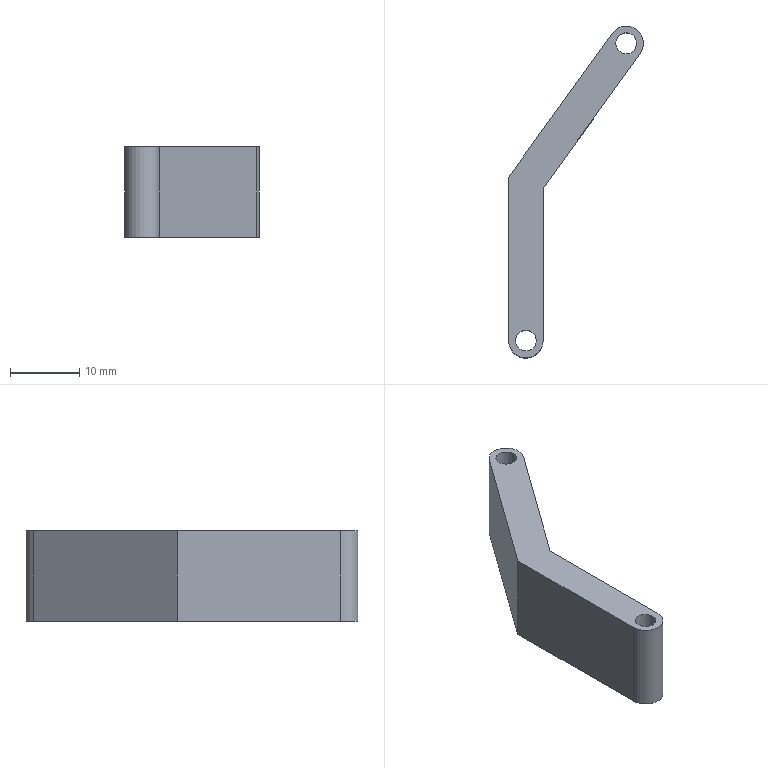Part | SolidWorks | features BaseBody 1 | 1 solid | 12 faces | box 19.494 x 47.938 x 13 mm | volume 3166 mm3 | cylinder 6 | plane 6 | commonest cylinder face diameters 3 x4 5 x2
STEP:
#1=CARTESIAN_POINT('',(-4.,-22.,13.));
#2=VERTEX_POINT('',#1);
#3=CARTESIAN_POINT('',(-1.,-22.,13.));
#4=VERTEX_POINT('',#3);
#5=CARTESIAN_POINT('',(-2.5,-22.,13.));
#6=DIRECTION('',(0.,0.,1.));
#7=DIRECTION('',(1.,0.,0.));
#8=AXIS2_PLACEMENT_3D('',#5,#6,#7);
#9=CIRCLE('',#8,1.5);
#10=EDGE_CURVE('',#2,#4,#9,.T.);
#11=ORIENTED_EDGE('',*,*,#10,.T.);
#12=CARTESIAN_POINT('',(-1.,-22.,0.));
#13=VERTEX_POINT('',#12);
#14=CARTESIAN_POINT('',(-1.,-22.,13.));
#15=DIRECTION('',(0.,0.,-1.));
#16=VECTOR('',#15,1000.);
#17=LINE('',#14,#16);
#18=EDGE_CURVE('',#4,#13,#17,.T.);
#19=ORIENTED_EDGE('',*,*,#18,.T.);
#20=CARTESIAN_POINT('',(-4.,-22.,0.));
#21=VERTEX_POINT('',#20);
#22=CARTESIAN_POINT('',(-2.5,-22.,0.));
#23=DIRECTION('',(0.,0.,1.));
#24=DIRECTION('',(1.,0.,0.));
#25=AXIS2_PLACEMENT_3D('',#22,#23,#24);
#26=CIRCLE('',#25,1.5);
#27=EDGE_CURVE('',#21,#13,#26,.T.);
#28=ORIENTED_EDGE('',*,*,#27,.F.);
#29=CARTESIAN_POINT('',(-4.,-22.,13.));
#30=DIRECTION('',(0.,0.,-1.));
#31=VECTOR('',#30,1000.);
#32=LINE('',#29,#31);
#33=EDGE_CURVE('',#2,#21,#32,.T.);
#34=ORIENTED_EDGE('',*,*,#33,.F.);
#35=EDGE_LOOP('',(#11,#19,#28,#34));
#36=FACE_OUTER_BOUND('',#35,.T.);
#37=CARTESIAN_POINT('',(-2.5,-22.,13.));
#38=DIRECTION('',(0.,0.,-1.));
#39=DIRECTION('',(-1.,0.,0.));
#40=AXIS2_PLACEMENT_3D('',#37,#38,#39);
#41=CYLINDRICAL_SURFACE('',#40,1.5);
#42=ADVANCED_FACE('',(#36),#41,.F.);
#43=CARTESIAN_POINT('',(10.494,20.938,13.));
#44=VERTEX_POINT('',#43);
#45=CARTESIAN_POINT('',(13.494,20.938,13.));
#46=VERTEX_POINT('',#45);
#47=CARTESIAN_POINT('',(11.994,20.938,13.));
#48=DIRECTION('',(0.,0.,1.));
#49=DIRECTION('',(1.,0.,0.));
#50=AXIS2_PLACEMENT_3D('',#47,#48,#49);
#51=CIRCLE('',#50,1.5);
#52=EDGE_CURVE('',#44,#46,#51,.T.);
#53=ORIENTED_EDGE('',*,*,#52,.T.);
#54=CARTESIAN_POINT('',(13.494,20.938,0.));
#55=VERTEX_POINT('',#54);
#56=CARTESIAN_POINT('',(13.494,20.938,13.));
#57=DIRECTION('',(0.,0.,-1.));
#58=VECTOR('',#57,1000.);
#59=LINE('',#56,#58);
#60=EDGE_CURVE('',#46,#55,#59,.T.);
#61=ORIENTED_EDGE('',*,*,#60,.T.);
#62=CARTESIAN_POINT('',(10.494,20.938,0.));
#63=VERTEX_POINT('',#62);
#64=CARTESIAN_POINT('',(11.994,20.938,0.));
#65=DIRECTION('',(0.,0.,1.));
#66=DIRECTION('',(1.,0.,0.));
#67=AXIS2_PLACEMENT_3D('',#64,#65,#66);
#68=CIRCLE('',#67,1.5);
#69=EDGE_CURVE('',#63,#55,#68,.T.);
#70=ORIENTED_EDGE('',*,*,#69,.F.);
#71=CARTESIAN_POINT('',(10.494,20.938,13.));
#72=DIRECTION('',(0.,0.,-1.));
#73=VECTOR('',#72,1000.);
#74=LINE('',#71,#73);
#75=EDGE_CURVE('',#44,#63,#74,.T.);
#76=ORIENTED_EDGE('',*,*,#75,.F.);
#77=EDGE_LOOP('',(#53,#61,#70,#76));
#78=FACE_OUTER_BOUND('',#77,.T.);
#79=CARTESIAN_POINT('',(11.994,20.938,13.));
#80=DIRECTION('',(0.,0.,-1.));
#81=DIRECTION('',(-1.,0.,0.));
#82=AXIS2_PLACEMENT_3D('',#79,#80,#81);
#83=CYLINDRICAL_SURFACE('',#82,1.5);
#84=ADVANCED_FACE('',(#78),#83,.F.);
#85=ORIENTED_EDGE('',*,*,#52,.F.);
#86=CARTESIAN_POINT('',(11.994,20.938,13.));
#87=DIRECTION('',(0.,0.,1.));
#88=DIRECTION('',(1.,0.,0.));
#89=AXIS2_PLACEMENT_3D('',#86,#87,#88);
#90=CIRCLE('',#89,1.5);
#91=EDGE_CURVE('',#46,#44,#90,.T.);
#92=ORIENTED_EDGE('',*,*,#91,.F.);
#93=EDGE_LOOP('',(#85,#92));
#94=FACE_BOUND('',#93,.T.);
#95=CARTESIAN_POINT('',(0.,0.,13.));
#96=VERTEX_POINT('',#95);
#97=CARTESIAN_POINT('',(14.023,19.477,13.));
#98=VERTEX_POINT('',#97);
#99=CARTESIAN_POINT('',(0.,0.,13.));
#100=DIRECTION('',(0.5843,0.8115,0.));
#101=VECTOR('',#100,1000.);
#102=LINE('',#99,#101);
#103=EDGE_CURVE('',#96,#98,#102,.T.);
#104=ORIENTED_EDGE('',*,*,#103,.T.);
#105=CARTESIAN_POINT('',(9.966,22.398,13.));
#106=VERTEX_POINT('',#105);
#107=CARTESIAN_POINT('',(11.994,20.938,13.));
#108=DIRECTION('',(0.,0.,1.));
#109=DIRECTION('',(1.,0.,0.));
#110=AXIS2_PLACEMENT_3D('',#107,#108,#109);
#111=CIRCLE('',#110,2.5);
#112=EDGE_CURVE('',#98,#106,#111,.T.);
#113=ORIENTED_EDGE('',*,*,#112,.T.);
#114=CARTESIAN_POINT('',(-5.,1.613,13.));
#115=VERTEX_POINT('',#114);
#116=CARTESIAN_POINT('',(-5.,1.613,13.));
#117=DIRECTION('',(-0.5843,-0.8115,0.));
#118=VECTOR('',#117,1000.);
#119=LINE('',#116,#118);
#120=EDGE_CURVE('',#106,#115,#119,.T.);
#121=ORIENTED_EDGE('',*,*,#120,.T.);
#122=CARTESIAN_POINT('',(-5.,-22.,13.));
#123=VERTEX_POINT('',#122);
#124=CARTESIAN_POINT('',(-5.,1.613,13.));
#125=DIRECTION('',(0.,-1.,0.));
#126=VECTOR('',#125,1000.);
#127=LINE('',#124,#126);
#128=EDGE_CURVE('',#115,#123,#127,.T.);
#129=ORIENTED_EDGE('',*,*,#128,.T.);
#130=CARTESIAN_POINT('',(0.,-22.,13.));
#131=VERTEX_POINT('',#130);
#132=CARTESIAN_POINT('',(-2.5,-22.,13.));
#133=DIRECTION('',(0.,0.,1.));
#134=DIRECTION('',(-1.,0.,0.));
#135=AXIS2_PLACEMENT_3D('',#132,#133,#134);
#136=CIRCLE('',#135,2.5);
#137=EDGE_CURVE('',#123,#131,#136,.T.);
#138=ORIENTED_EDGE('',*,*,#137,.T.);
#139=CARTESIAN_POINT('',(0.,0.,13.));
#140=DIRECTION('',(0.,1.,0.));
#141=VECTOR('',#140,1000.);
#142=LINE('',#139,#141);
#143=EDGE_CURVE('',#131,#96,#142,.T.);
#144=ORIENTED_EDGE('',*,*,#143,.T.);
#145=EDGE_LOOP('',(#104,#113,#121,#129,#138,#144));
#146=FACE_OUTER_BOUND('',#145,.T.);
#147=ORIENTED_EDGE('',*,*,#10,.F.);
#148=CARTESIAN_POINT('',(-2.5,-22.,13.));
#149=DIRECTION('',(0.,0.,1.));
#150=DIRECTION('',(1.,0.,0.));
#151=AXIS2_PLACEMENT_3D('',#148,#149,#150);
#152=CIRCLE('',#151,1.5);
#153=EDGE_CURVE('',#4,#2,#152,.T.);
#154=ORIENTED_EDGE('',*,*,#153,.F.);
#155=EDGE_LOOP('',(#147,#154));
#156=FACE_BOUND('',#155,.T.);
#157=CARTESIAN_POINT('',(11.994,20.938,13.));
#158=DIRECTION('',(0.,0.,1.));
#159=DIRECTION('',(1.,0.,0.));
#160=AXIS2_PLACEMENT_3D('',#157,#158,#159);
#161=PLANE('',#160);
#162=ADVANCED_FACE('',(#94,#146,#156),#161,.T.);
#163=CARTESIAN_POINT('',(0.,0.,0.));
#164=VERTEX_POINT('',#163);
#165=CARTESIAN_POINT('',(14.023,19.477,0.));
#166=VERTEX_POINT('',#165);
#167=CARTESIAN_POINT('',(0.,0.,0.));
#168=DIRECTION('',(0.5843,0.8115,0.));
#169=VECTOR('',#168,1000.);
#170=LINE('',#167,#169);
#171=EDGE_CURVE('',#164,#166,#170,.T.);
#172=ORIENTED_EDGE('',*,*,#171,.F.);
#173=CARTESIAN_POINT('',(0.,-22.,0.));
#174=VERTEX_POINT('',#173);
#175=CARTESIAN_POINT('',(0.,0.,0.));
#176=DIRECTION('',(0.,1.,0.));
#177=VECTOR('',#176,1000.);
#178=LINE('',#175,#177);
#179=EDGE_CURVE('',#174,#164,#178,.T.);
#180=ORIENTED_EDGE('',*,*,#179,.F.);
#181=CARTESIAN_POINT('',(-5.,-22.,0.));
#182=VERTEX_POINT('',#181);
#183=CARTESIAN_POINT('',(-2.5,-22.,0.));
#184=DIRECTION('',(0.,0.,1.));
#185=DIRECTION('',(-1.,0.,0.));
#186=AXIS2_PLACEMENT_3D('',#183,#184,#185);
#187=CIRCLE('',#186,2.5);
#188=EDGE_CURVE('',#182,#174,#187,.T.);
#189=ORIENTED_EDGE('',*,*,#188,.F.);
#190=CARTESIAN_POINT('',(-5.,1.613,0.));
#191=VERTEX_POINT('',#190);
#192=CARTESIAN_POINT('',(-5.,1.613,0.));
#193=DIRECTION('',(0.,-1.,0.));
#194=VECTOR('',#193,1000.);
#195=LINE('',#192,#194);
#196=EDGE_CURVE('',#191,#182,#195,.T.);
#197=ORIENTED_EDGE('',*,*,#196,.F.);
#198=CARTESIAN_POINT('',(9.966,22.398,0.));
#199=VERTEX_POINT('',#198);
#200=CARTESIAN_POINT('',(-5.,1.613,0.));
#201=DIRECTION('',(-0.5843,-0.8115,0.));
#202=VECTOR('',#201,1000.);
#203=LINE('',#200,#202);
#204=EDGE_CURVE('',#199,#191,#203,.T.);
#205=ORIENTED_EDGE('',*,*,#204,.F.);
#206=CARTESIAN_POINT('',(11.994,20.938,0.));
#207=DIRECTION('',(0.,0.,1.));
#208=DIRECTION('',(1.,0.,0.));
#209=AXIS2_PLACEMENT_3D('',#206,#207,#208);
#210=CIRCLE('',#209,2.5);
#211=EDGE_CURVE('',#166,#199,#210,.T.);
#212=ORIENTED_EDGE('',*,*,#211,.F.);
#213=EDGE_LOOP('',(#172,#180,#189,#197,#205,#212));
#214=FACE_OUTER_BOUND('',#213,.T.);
#215=ORIENTED_EDGE('',*,*,#69,.T.);
#216=CARTESIAN_POINT('',(11.994,20.938,0.));
#217=DIRECTION('',(0.,0.,1.));
#218=DIRECTION('',(1.,0.,0.));
#219=AXIS2_PLACEMENT_3D('',#216,#217,#218);
#220=CIRCLE('',#219,1.5);
#221=EDGE_CURVE('',#55,#63,#220,.T.);
#222=ORIENTED_EDGE('',*,*,#221,.T.);
#223=EDGE_LOOP('',(#215,#222));
#224=FACE_BOUND('',#223,.T.);
#225=ORIENTED_EDGE('',*,*,#27,.T.);
#226=CARTESIAN_POINT('',(-2.5,-22.,0.));
#227=DIRECTION('',(0.,0.,1.));
#228=DIRECTION('',(1.,0.,0.));
#229=AXIS2_PLACEMENT_3D('',#226,#227,#228);
#230=CIRCLE('',#229,1.5);
#231=EDGE_CURVE('',#13,#21,#230,.T.);
#232=ORIENTED_EDGE('',*,*,#231,.T.);
#233=EDGE_LOOP('',(#225,#232));
#234=FACE_BOUND('',#233,.T.);
#235=CARTESIAN_POINT('',(11.994,20.938,0.));
#236=DIRECTION('',(0.,0.,1.));
#237=DIRECTION('',(1.,0.,0.));
#238=AXIS2_PLACEMENT_3D('',#235,#236,#237);
#239=PLANE('',#238);
#240=ADVANCED_FACE('',(#214,#224,#234),#239,.F.);
#241=ORIENTED_EDGE('',*,*,#171,.T.);
#242=CARTESIAN_POINT('',(14.023,19.477,13.));
#243=DIRECTION('',(0.,0.,-1.));
#244=VECTOR('',#243,1000.);
#245=LINE('',#242,#244);
#246=EDGE_CURVE('',#98,#166,#245,.T.);
#247=ORIENTED_EDGE('',*,*,#246,.F.);
#248=ORIENTED_EDGE('',*,*,#103,.F.);
#249=CARTESIAN_POINT('',(0.,0.,13.));
#250=DIRECTION('',(0.,0.,-1.));
#251=VECTOR('',#250,1000.);
#252=LINE('',#249,#251);
#253=EDGE_CURVE('',#96,#164,#252,.T.);
#254=ORIENTED_EDGE('',*,*,#253,.T.);
#255=EDGE_LOOP('',(#241,#247,#248,#254));
#256=FACE_OUTER_BOUND('',#255,.T.);
#257=CARTESIAN_POINT('',(0.,0.,13.));
#258=DIRECTION('',(-0.8115,0.5843,0.));
#259=DIRECTION('',(-0.5843,-0.8115,0.));
#260=AXIS2_PLACEMENT_3D('',#257,#258,#259);
#261=PLANE('',#260);
#262=ADVANCED_FACE('',(#256),#261,.F.);
#263=ORIENTED_EDGE('',*,*,#211,.T.);
#264=CARTESIAN_POINT('',(9.966,22.398,13.));
#265=DIRECTION('',(0.,0.,-1.));
#266=VECTOR('',#265,1000.);
#267=LINE('',#264,#266);
#268=EDGE_CURVE('',#106,#199,#267,.T.);
#269=ORIENTED_EDGE('',*,*,#268,.F.);
#270=ORIENTED_EDGE('',*,*,#112,.F.);
#271=ORIENTED_EDGE('',*,*,#246,.T.);
#272=EDGE_LOOP('',(#263,#269,#270,#271));
#273=FACE_OUTER_BOUND('',#272,.T.);
#274=CARTESIAN_POINT('',(11.994,20.938,13.));
#275=DIRECTION('',(0.,0.,-1.));
#276=DIRECTION('',(-1.,0.,0.));
#277=AXIS2_PLACEMENT_3D('',#274,#275,#276);
#278=CYLINDRICAL_SURFACE('',#277,2.5);
#279=ADVANCED_FACE('',(#273),#278,.T.);
#280=ORIENTED_EDGE('',*,*,#204,.T.);
#281=CARTESIAN_POINT('',(-5.,1.613,13.));
#282=DIRECTION('',(0.,0.,-1.));
#283=VECTOR('',#282,1000.);
#284=LINE('',#281,#283);
#285=EDGE_CURVE('',#115,#191,#284,.T.);
#286=ORIENTED_EDGE('',*,*,#285,.F.);
#287=ORIENTED_EDGE('',*,*,#120,.F.);
#288=ORIENTED_EDGE('',*,*,#268,.T.);
#289=EDGE_LOOP('',(#280,#286,#287,#288));
#290=FACE_OUTER_BOUND('',#289,.T.);
#291=CARTESIAN_POINT('',(-5.,1.613,13.));
#292=DIRECTION('',(0.8115,-0.5843,0.));
#293=DIRECTION('',(0.5843,0.8115,0.));
#294=AXIS2_PLACEMENT_3D('',#291,#292,#293);
#295=PLANE('',#294);
#296=ADVANCED_FACE('',(#290),#295,.F.);
#297=ORIENTED_EDGE('',*,*,#196,.T.);
#298=CARTESIAN_POINT('',(-5.,-22.,13.));
#299=DIRECTION('',(0.,0.,-1.));
#300=VECTOR('',#299,1000.);
#301=LINE('',#298,#300);
#302=EDGE_CURVE('',#123,#182,#301,.T.);
#303=ORIENTED_EDGE('',*,*,#302,.F.);
#304=ORIENTED_EDGE('',*,*,#128,.F.);
#305=ORIENTED_EDGE('',*,*,#285,.T.);
#306=EDGE_LOOP('',(#297,#303,#304,#305));
#307=FACE_OUTER_BOUND('',#306,.T.);
#308=CARTESIAN_POINT('',(-5.,1.613,13.));
#309=DIRECTION('',(1.,0.,0.));
#310=DIRECTION('',(0.,1.,0.));
#311=AXIS2_PLACEMENT_3D('',#308,#309,#310);
#312=PLANE('',#311);
#313=ADVANCED_FACE('',(#307),#312,.F.);
#314=ORIENTED_EDGE('',*,*,#188,.T.);
#315=CARTESIAN_POINT('',(0.,-22.,13.));
#316=DIRECTION('',(0.,0.,-1.));
#317=VECTOR('',#316,1000.);
#318=LINE('',#315,#317);
#319=EDGE_CURVE('',#131,#174,#318,.T.);
#320=ORIENTED_EDGE('',*,*,#319,.F.);
#321=ORIENTED_EDGE('',*,*,#137,.F.);
#322=ORIENTED_EDGE('',*,*,#302,.T.);
#323=EDGE_LOOP('',(#314,#320,#321,#322));
#324=FACE_OUTER_BOUND('',#323,.T.);
#325=CARTESIAN_POINT('',(-2.5,-22.,13.));
#326=DIRECTION('',(0.,0.,-1.));
#327=DIRECTION('',(-1.,0.,0.));
#328=AXIS2_PLACEMENT_3D('',#325,#326,#327);
#329=CYLINDRICAL_SURFACE('',#328,2.5);
#330=ADVANCED_FACE('',(#324),#329,.T.);
#331=ORIENTED_EDGE('',*,*,#179,.T.);
#332=ORIENTED_EDGE('',*,*,#253,.F.);
#333=ORIENTED_EDGE('',*,*,#143,.F.);
#334=ORIENTED_EDGE('',*,*,#319,.T.);
#335=EDGE_LOOP('',(#331,#332,#333,#334));
#336=FACE_OUTER_BOUND('',#335,.T.);
#337=CARTESIAN_POINT('',(0.,0.,13.));
#338=DIRECTION('',(-1.,0.,0.));
#339=DIRECTION('',(0.,-1.,0.));
#340=AXIS2_PLACEMENT_3D('',#337,#338,#339);
#341=PLANE('',#340);
#342=ADVANCED_FACE('',(#336),#341,.F.);
#343=ORIENTED_EDGE('',*,*,#60,.F.);
#344=ORIENTED_EDGE('',*,*,#91,.T.);
#345=ORIENTED_EDGE('',*,*,#75,.T.);
#346=ORIENTED_EDGE('',*,*,#221,.F.);
#347=EDGE_LOOP('',(#343,#344,#345,#346));
#348=FACE_OUTER_BOUND('',#347,.T.);
#349=CARTESIAN_POINT('',(11.994,20.938,13.));
#350=DIRECTION('',(0.,0.,-1.));
#351=DIRECTION('',(-1.,0.,0.));
#352=AXIS2_PLACEMENT_3D('',#349,#350,#351);
#353=CYLINDRICAL_SURFACE('',#352,1.5);
#354=ADVANCED_FACE('',(#348),#353,.F.);
#355=ORIENTED_EDGE('',*,*,#18,.F.);
#356=ORIENTED_EDGE('',*,*,#153,.T.);
#357=ORIENTED_EDGE('',*,*,#33,.T.);
#358=ORIENTED_EDGE('',*,*,#231,.F.);
#359=EDGE_LOOP('',(#355,#356,#357,#358));
#360=FACE_OUTER_BOUND('',#359,.T.);
#361=CARTESIAN_POINT('',(-2.5,-22.,13.));
#362=DIRECTION('',(0.,0.,-1.));
#363=DIRECTION('',(-1.,0.,0.));
#364=AXIS2_PLACEMENT_3D('',#361,#362,#363);
#365=CYLINDRICAL_SURFACE('',#364,1.5);
#366=ADVANCED_FACE('',(#360),#365,.F.);
#367=CLOSED_SHELL('',(#42,#84,#162,#240,#262,#279,#296,#313,#330,#342,#354,#366));
#368=MANIFOLD_SOLID_BREP('',#367);
#369=CARTESIAN_POINT('',(0.,0.,0.));
#370=DIRECTION('',(0.,0.,1.));
#371=DIRECTION('',(1.,0.,0.));
#372=AXIS2_PLACEMENT_3D('',#369,#370,#371);
#373=(LENGTH_UNIT()NAMED_UNIT(*)SI_UNIT(.MILLI.,.METRE.));
#374=UNCERTAINTY_MEASURE_WITH_UNIT(LENGTH_MEASURE(0.00001),#373,'','');
#375=(NAMED_UNIT(*)PLANE_ANGLE_UNIT()SI_UNIT($,.RADIAN.));
#376=(NAMED_UNIT(*)SI_UNIT($,.STERADIAN.)SOLID_ANGLE_UNIT());
#377=(GEOMETRIC_REPRESENTATION_CONTEXT(3)GLOBAL_UNCERTAINTY_ASSIGNED_CONTEXT((#374))GLOBAL_UNIT_ASSIGNED_CONTEXT((#373,#375,#376))REPRESENTATION_CONTEXT('',''));
#378=ADVANCED_BREP_SHAPE_REPRESENTATION('',(#368,#372),#377);